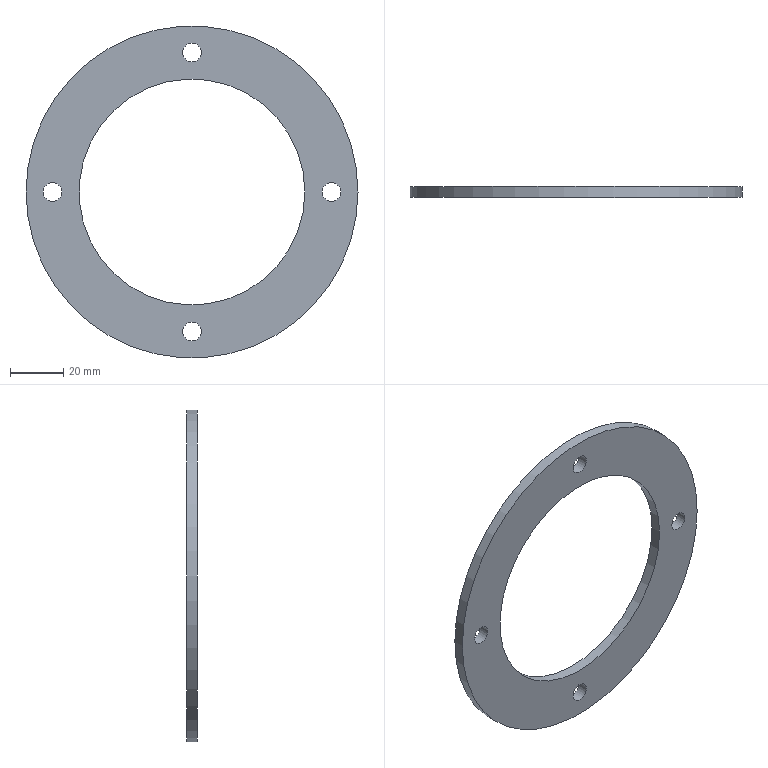Part | NX | features DATUM_CSYS 2, EXTRUDE 1, SKETCH 1 | 1 solid | 8 faces | box 125 x 4 x 125 mm | volume 25774 mm3 | cylinder 6 | plane 2 | commonest cylinder face diameters 7 x4 85 x1 125 x1
STEP:
#1=CARTESIAN_POINT('',(-3.5,-4.,-52.5));
#2=VERTEX_POINT('',#1);
#3=CARTESIAN_POINT('',(0.,-4.,-52.5));
#4=DIRECTION('',(0.,-1.,0.));
#5=DIRECTION('',(-1.,0.,0.));
#6=AXIS2_PLACEMENT_3D('',#3,#4,#5);
#7=CIRCLE('',#6,3.5);
#8=EDGE_CURVE('',#2,#2,#7,.T.);
#9=ORIENTED_EDGE('',*,*,#8,.T.);
#10=EDGE_LOOP('',(#9));
#11=FACE_BOUND('',#10,.T.);
#12=CARTESIAN_POINT('',(-3.5,0.,-52.5));
#13=VERTEX_POINT('',#12);
#14=CARTESIAN_POINT('',(0.,0.,-52.5));
#15=DIRECTION('',(0.,-1.,0.));
#16=DIRECTION('',(-1.,0.,0.));
#17=AXIS2_PLACEMENT_3D('',#14,#15,#16);
#18=CIRCLE('',#17,3.5);
#19=EDGE_CURVE('',#13,#13,#18,.T.);
#20=ORIENTED_EDGE('',*,*,#19,.F.);
#21=EDGE_LOOP('',(#20));
#22=FACE_BOUND('',#21,.T.);
#23=CARTESIAN_POINT('',(0.,-4.,-52.5));
#24=DIRECTION('',(0.,1.,0.));
#25=DIRECTION('',(0.,0.,1.));
#26=AXIS2_PLACEMENT_3D('',#23,#24,#25);
#27=CYLINDRICAL_SURFACE('',#26,3.5);
#28=ADVANCED_FACE('',(#11,#22),#27,.F.);
#29=CARTESIAN_POINT('',(-52.5,-4.,3.5));
#30=VERTEX_POINT('',#29);
#31=CARTESIAN_POINT('',(-52.5,-4.,0.));
#32=DIRECTION('',(0.,-1.,0.));
#33=DIRECTION('',(0.,0.,1.));
#34=AXIS2_PLACEMENT_3D('',#31,#32,#33);
#35=CIRCLE('',#34,3.5);
#36=EDGE_CURVE('',#30,#30,#35,.T.);
#37=ORIENTED_EDGE('',*,*,#36,.T.);
#38=EDGE_LOOP('',(#37));
#39=FACE_BOUND('',#38,.T.);
#40=CARTESIAN_POINT('',(-52.5,0.,3.5));
#41=VERTEX_POINT('',#40);
#42=CARTESIAN_POINT('',(-52.5,0.,0.));
#43=DIRECTION('',(0.,-1.,0.));
#44=DIRECTION('',(0.,0.,1.));
#45=AXIS2_PLACEMENT_3D('',#42,#43,#44);
#46=CIRCLE('',#45,3.5);
#47=EDGE_CURVE('',#41,#41,#46,.T.);
#48=ORIENTED_EDGE('',*,*,#47,.F.);
#49=EDGE_LOOP('',(#48));
#50=FACE_BOUND('',#49,.T.);
#51=CARTESIAN_POINT('',(-52.5,-4.,0.));
#52=DIRECTION('',(0.,1.,0.));
#53=DIRECTION('',(0.,0.,1.));
#54=AXIS2_PLACEMENT_3D('',#51,#52,#53);
#55=CYLINDRICAL_SURFACE('',#54,3.5);
#56=ADVANCED_FACE('',(#39,#50),#55,.F.);
#57=CARTESIAN_POINT('',(42.5,-4.,0.));
#58=VERTEX_POINT('',#57);
#59=CARTESIAN_POINT('',(0.,-4.,0.));
#60=DIRECTION('',(0.,-1.,0.));
#61=DIRECTION('',(1.,0.,0.));
#62=AXIS2_PLACEMENT_3D('',#59,#60,#61);
#63=CIRCLE('',#62,42.5);
#64=EDGE_CURVE('',#58,#58,#63,.T.);
#65=ORIENTED_EDGE('',*,*,#64,.T.);
#66=EDGE_LOOP('',(#65));
#67=FACE_BOUND('',#66,.T.);
#68=CARTESIAN_POINT('',(42.5,0.,0.));
#69=VERTEX_POINT('',#68);
#70=CARTESIAN_POINT('',(0.,0.,0.));
#71=DIRECTION('',(0.,-1.,0.));
#72=DIRECTION('',(1.,0.,0.));
#73=AXIS2_PLACEMENT_3D('',#70,#71,#72);
#74=CIRCLE('',#73,42.5);
#75=EDGE_CURVE('',#69,#69,#74,.T.);
#76=ORIENTED_EDGE('',*,*,#75,.F.);
#77=EDGE_LOOP('',(#76));
#78=FACE_BOUND('',#77,.T.);
#79=CARTESIAN_POINT('',(0.,-4.,0.));
#80=DIRECTION('',(0.,1.,0.));
#81=DIRECTION('',(0.,0.,1.));
#82=AXIS2_PLACEMENT_3D('',#79,#80,#81);
#83=CYLINDRICAL_SURFACE('',#82,42.5);
#84=ADVANCED_FACE('',(#67,#78),#83,.F.);
#85=CARTESIAN_POINT('',(3.5,-4.,52.5));
#86=VERTEX_POINT('',#85);
#87=CARTESIAN_POINT('',(0.,-4.,52.5));
#88=DIRECTION('',(0.,-1.,0.));
#89=DIRECTION('',(1.,0.,0.));
#90=AXIS2_PLACEMENT_3D('',#87,#88,#89);
#91=CIRCLE('',#90,3.5);
#92=EDGE_CURVE('',#86,#86,#91,.T.);
#93=ORIENTED_EDGE('',*,*,#92,.T.);
#94=EDGE_LOOP('',(#93));
#95=FACE_BOUND('',#94,.T.);
#96=CARTESIAN_POINT('',(3.5,0.,52.5));
#97=VERTEX_POINT('',#96);
#98=CARTESIAN_POINT('',(0.,0.,52.5));
#99=DIRECTION('',(0.,-1.,0.));
#100=DIRECTION('',(1.,0.,0.));
#101=AXIS2_PLACEMENT_3D('',#98,#99,#100);
#102=CIRCLE('',#101,3.5);
#103=EDGE_CURVE('',#97,#97,#102,.T.);
#104=ORIENTED_EDGE('',*,*,#103,.F.);
#105=EDGE_LOOP('',(#104));
#106=FACE_BOUND('',#105,.T.);
#107=CARTESIAN_POINT('',(0.,-4.,52.5));
#108=DIRECTION('',(0.,1.,0.));
#109=DIRECTION('',(0.,0.,1.));
#110=AXIS2_PLACEMENT_3D('',#107,#108,#109);
#111=CYLINDRICAL_SURFACE('',#110,3.5);
#112=ADVANCED_FACE('',(#95,#106),#111,.F.);
#113=CARTESIAN_POINT('',(62.5,-4.,0.));
#114=VERTEX_POINT('',#113);
#115=CARTESIAN_POINT('',(0.,-4.,0.));
#116=DIRECTION('',(0.,-1.,0.));
#117=DIRECTION('',(1.,0.,0.));
#118=AXIS2_PLACEMENT_3D('',#115,#116,#117);
#119=CIRCLE('',#118,62.5);
#120=EDGE_CURVE('',#114,#114,#119,.T.);
#121=ORIENTED_EDGE('',*,*,#120,.F.);
#122=EDGE_LOOP('',(#121));
#123=FACE_BOUND('',#122,.T.);
#124=CARTESIAN_POINT('',(62.5,0.,0.));
#125=VERTEX_POINT('',#124);
#126=CARTESIAN_POINT('',(0.,0.,0.));
#127=DIRECTION('',(0.,-1.,0.));
#128=DIRECTION('',(1.,0.,0.));
#129=AXIS2_PLACEMENT_3D('',#126,#127,#128);
#130=CIRCLE('',#129,62.5);
#131=EDGE_CURVE('',#125,#125,#130,.T.);
#132=ORIENTED_EDGE('',*,*,#131,.T.);
#133=EDGE_LOOP('',(#132));
#134=FACE_BOUND('',#133,.T.);
#135=CARTESIAN_POINT('',(0.,-4.,0.));
#136=DIRECTION('',(0.,1.,0.));
#137=DIRECTION('',(0.,0.,1.));
#138=AXIS2_PLACEMENT_3D('',#135,#136,#137);
#139=CYLINDRICAL_SURFACE('',#138,62.5);
#140=ADVANCED_FACE('',(#123,#134),#139,.T.);
#141=CARTESIAN_POINT('',(52.5,-4.,-3.5));
#142=VERTEX_POINT('',#141);
#143=CARTESIAN_POINT('',(52.5,-4.,0.));
#144=DIRECTION('',(0.,-1.,0.));
#145=DIRECTION('',(0.,0.,-1.));
#146=AXIS2_PLACEMENT_3D('',#143,#144,#145);
#147=CIRCLE('',#146,3.5);
#148=EDGE_CURVE('',#142,#142,#147,.T.);
#149=ORIENTED_EDGE('',*,*,#148,.T.);
#150=EDGE_LOOP('',(#149));
#151=FACE_BOUND('',#150,.T.);
#152=CARTESIAN_POINT('',(52.5,0.,-3.5));
#153=VERTEX_POINT('',#152);
#154=CARTESIAN_POINT('',(52.5,0.,0.));
#155=DIRECTION('',(0.,-1.,0.));
#156=DIRECTION('',(0.,0.,-1.));
#157=AXIS2_PLACEMENT_3D('',#154,#155,#156);
#158=CIRCLE('',#157,3.5);
#159=EDGE_CURVE('',#153,#153,#158,.T.);
#160=ORIENTED_EDGE('',*,*,#159,.F.);
#161=EDGE_LOOP('',(#160));
#162=FACE_BOUND('',#161,.T.);
#163=CARTESIAN_POINT('',(52.5,-4.,0.));
#164=DIRECTION('',(0.,1.,0.));
#165=DIRECTION('',(0.,0.,1.));
#166=AXIS2_PLACEMENT_3D('',#163,#164,#165);
#167=CYLINDRICAL_SURFACE('',#166,3.5);
#168=ADVANCED_FACE('',(#151,#162),#167,.F.);
#169=ORIENTED_EDGE('',*,*,#120,.T.);
#170=EDGE_LOOP('',(#169));
#171=FACE_BOUND('',#170,.T.);
#172=ORIENTED_EDGE('',*,*,#92,.F.);
#173=EDGE_LOOP('',(#172));
#174=FACE_BOUND('',#173,.T.);
#175=ORIENTED_EDGE('',*,*,#64,.F.);
#176=EDGE_LOOP('',(#175));
#177=FACE_BOUND('',#176,.T.);
#178=ORIENTED_EDGE('',*,*,#36,.F.);
#179=EDGE_LOOP('',(#178));
#180=FACE_BOUND('',#179,.T.);
#181=ORIENTED_EDGE('',*,*,#8,.F.);
#182=EDGE_LOOP('',(#181));
#183=FACE_BOUND('',#182,.T.);
#184=ORIENTED_EDGE('',*,*,#148,.F.);
#185=EDGE_LOOP('',(#184));
#186=FACE_BOUND('',#185,.T.);
#187=CARTESIAN_POINT('',(0.,-4.,26.25));
#188=DIRECTION('',(0.,-1.,0.));
#189=DIRECTION('',(0.,0.,-1.));
#190=AXIS2_PLACEMENT_3D('',#187,#188,#189);
#191=PLANE('',#190);
#192=ADVANCED_FACE('',(#171,#174,#177,#180,#183,#186),#191,.T.);
#193=ORIENTED_EDGE('',*,*,#131,.F.);
#194=EDGE_LOOP('',(#193));
#195=FACE_BOUND('',#194,.T.);
#196=ORIENTED_EDGE('',*,*,#103,.T.);
#197=EDGE_LOOP('',(#196));
#198=FACE_BOUND('',#197,.T.);
#199=ORIENTED_EDGE('',*,*,#75,.T.);
#200=EDGE_LOOP('',(#199));
#201=FACE_BOUND('',#200,.T.);
#202=ORIENTED_EDGE('',*,*,#47,.T.);
#203=EDGE_LOOP('',(#202));
#204=FACE_BOUND('',#203,.T.);
#205=ORIENTED_EDGE('',*,*,#19,.T.);
#206=EDGE_LOOP('',(#205));
#207=FACE_BOUND('',#206,.T.);
#208=ORIENTED_EDGE('',*,*,#159,.T.);
#209=EDGE_LOOP('',(#208));
#210=FACE_BOUND('',#209,.T.);
#211=CARTESIAN_POINT('',(0.,0.,26.25));
#212=DIRECTION('',(0.,-1.,0.));
#213=DIRECTION('',(0.,0.,-1.));
#214=AXIS2_PLACEMENT_3D('',#211,#212,#213);
#215=PLANE('',#214);
#216=ADVANCED_FACE('',(#195,#198,#201,#204,#207,#210),#215,.F.);
#217=CLOSED_SHELL('',(#28,#56,#84,#112,#140,#168,#192,#216));
#218=MANIFOLD_SOLID_BREP('',#217);
#219=(LENGTH_UNIT()NAMED_UNIT(*)SI_UNIT(.MILLI.,.METRE.));
#220=UNCERTAINTY_MEASURE_WITH_UNIT(LENGTH_MEASURE(0.00001),#219,'','');
#221=(NAMED_UNIT(*)PLANE_ANGLE_UNIT()SI_UNIT($,.RADIAN.));
#222=(NAMED_UNIT(*)SI_UNIT($,.STERADIAN.)SOLID_ANGLE_UNIT());
#223=(GEOMETRIC_REPRESENTATION_CONTEXT(3)GLOBAL_UNCERTAINTY_ASSIGNED_CONTEXT((#220))GLOBAL_UNIT_ASSIGNED_CONTEXT((#219,#221,#222))REPRESENTATION_CONTEXT('',''));
#224=ADVANCED_BREP_SHAPE_REPRESENTATION('',(#218),#223);